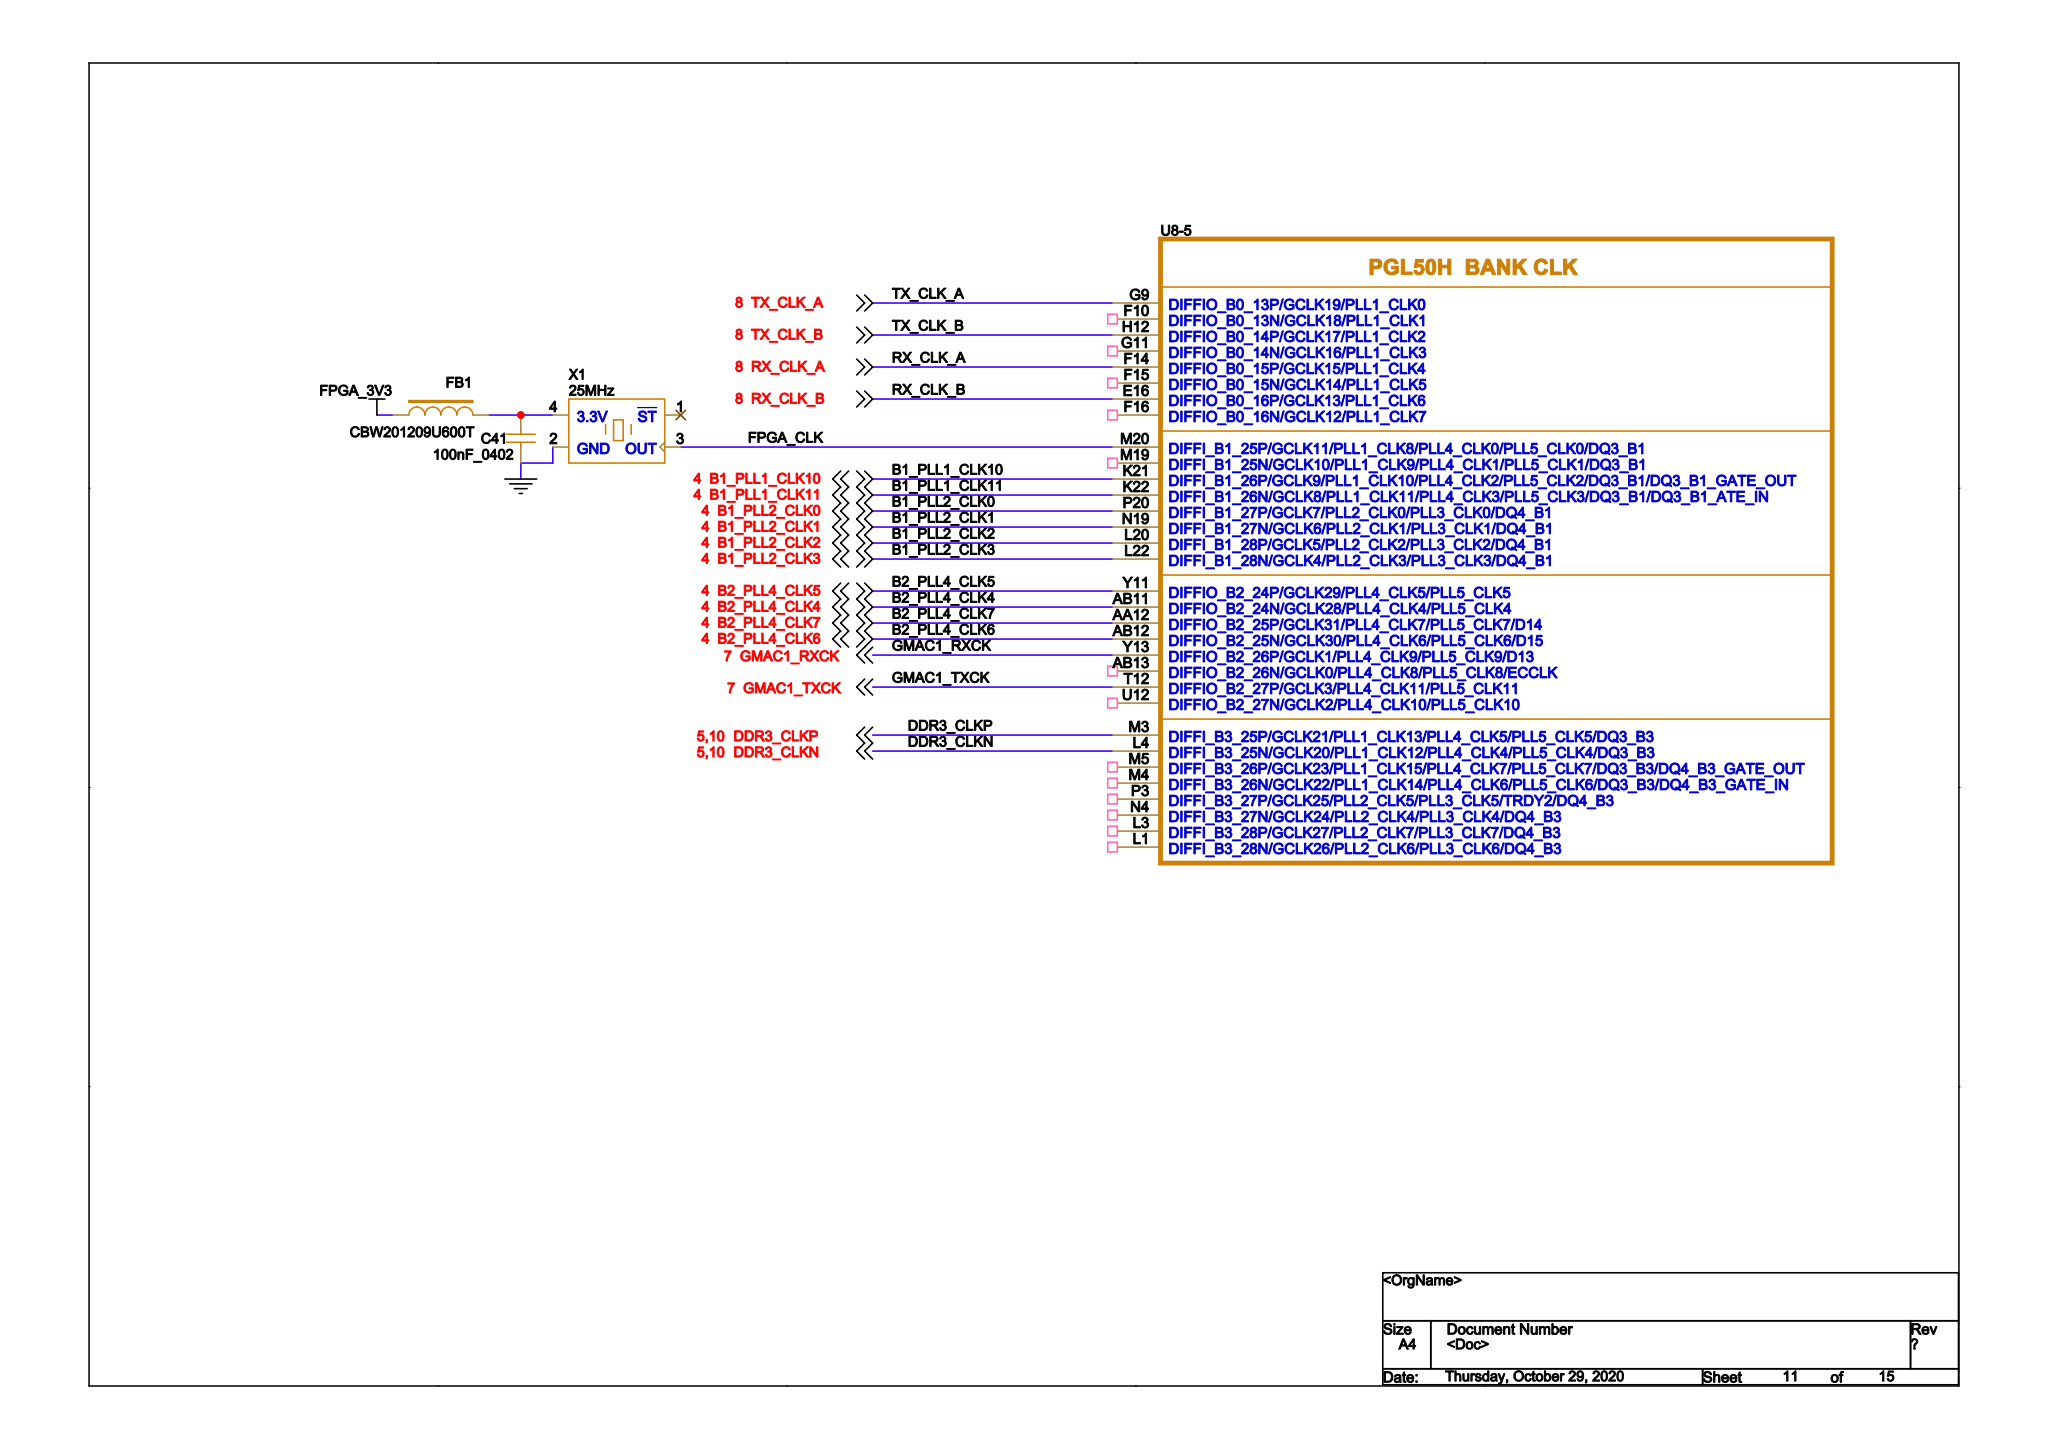Circuit board | Cadence Allegro | 406 parts | 392 nets | one sheet of the schematic
Parts on this sheet (reference | value | footprint):
C41 | 100nF_0402 | C_0402_104
FB1 | CBW201209U600T | L_0805
X1 | 25MHz | XTAL3225
Nets of these parts (net: part-pin ...):
GND: C41-2 X1-2
N20041801: C41-1 FB1-2 X1-4
FPGA_3V3: FB1-1
FPGA_CLK: X1-3